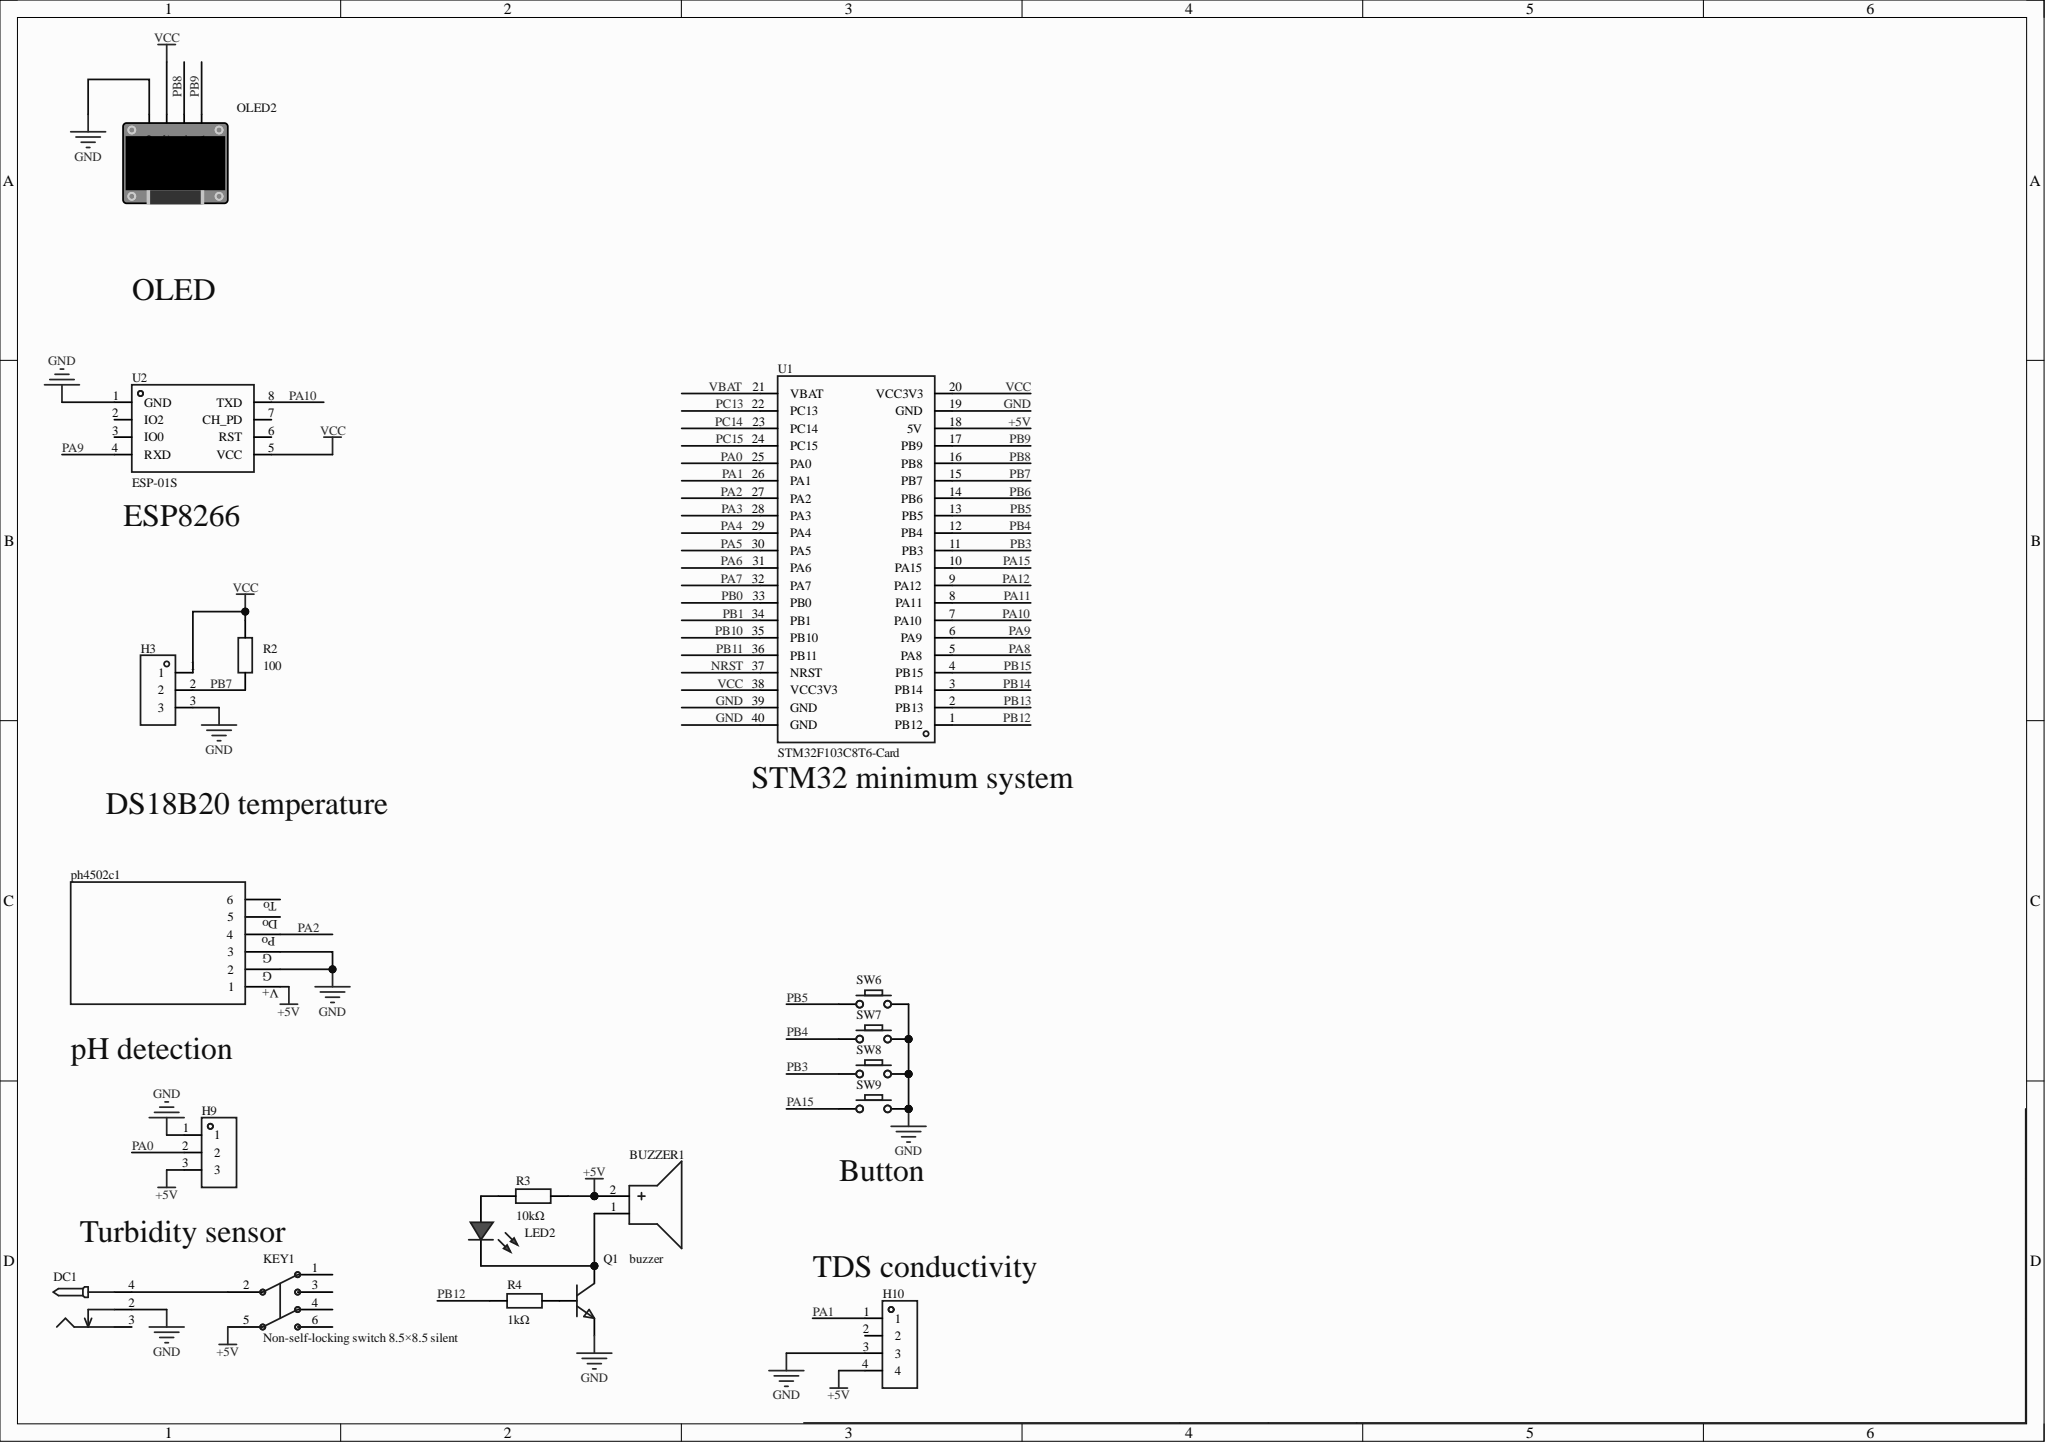Circuit board | Altium Designer | 19 parts | 20 nets
Bill of materials:
Comment,Description,Designator,Footprint,LibRef,Quantity
"buzzer","","BUZZER1","BUZ-TH_BD12.0-P6.00-D0.9-RD","buzzer","1"
"","","DC1","DC-2.0","DC-005_2.0","1"
"","","H3, H9","HDR-TH_3P-P2.54-V-F","HDR-F_2.54_1x3P","2"
"","","H10","HDR-TH_4P-P2.54-V-F","HDR-F_2.54_1x4P","1"
"Non-self-locking switch 8.5×8.5 silent","6脚，8.5×8.5","KEY1","SW-TH_6P-L8.5-W8.5-P2.54","无自锁开关 8.5×8.5 无声","1"
"","","LED2","LED_TH-3mm","LED_TH-R_3mm","1"
"","","OLED2","0.96OLED_4P","0.96OLED模块_4P","1"
"","","ph4502c1","PH4502C","PH4502C","1"
"","","Q1","S8050_TO_92","S8050_TO_NPN","1"
"100","","R2","Res_1/8W","Res_AXIAL-1/8W","1"
"10kΩ","","R3","Res_1/8W","Res_AXIAL-1/8W","1"
"1kΩ","","R4","Res_1/8W","Res_AXIAL-1/8W","1"
"","","SW6, SW7, SW8, SW9","Key_TH_3.5x6x4.3","Key_TH_3.5x6x4.3","4"
"STM32F103C8T6-Card","","U1","CONN-TH_L53.3-W22.9_STM32F103C8T6-CARD","STM32F103C8T6-Card","1"
"ESP-01S","","U2","WIFIM-TH_ESP-01S","ESP-01S_C111009","1"
Netlist (Protel format):
[
BUZZER1
BUZ-TH_BD12.0-P6.00-D0.9-RD
buzzer



]
[
DC1
DC-2.0




]
[
H3
HDR-TH_3P-P2.54-V-F




]
[
H9
HDR-TH_3P-P2.54-V-F




]
[
H10
HDR-TH_4P-P2.54-V-F




]
[
KEY1
SW-TH_6P-L8.5-W8.5-P2.54
Non-self-locking switch 8.5×8.5 silent



]
[
LED2
LED_TH-3mm




]
[
OLED2
0.96OLED_4P




]
[
ph4502c1
PH4502C




]
[
Q1
S8050_TO_92




]
[
R2
Res_1/8W
100



]
[
R3
Res_1/8W
10kΩ



]
[
R4
Res_1/8W
1kΩ



]
[
SW6
Key_TH_3.5x6x4.3




]
[
SW7
Key_TH_3.5x6x4.3




]
[
SW8
Key_TH_3.5x6x4.3




]
[
SW9
Key_TH_3.5x6x4.3




]
[
U1
CONN-TH_L53.3-W22.9_STM32F103C8T6-CARD
STM32F103C8T6-Card



]
[
U2
WIFIM-TH_ESP-01S
ESP-01S



]
(
VCC
H3-1
OLED2-2
R2-2
U1-20
U1-38
U2-5
)
(
PB12
R4-1
U1-1
)
(
PB9
OLED2-4
U1-17
)
(
PB8
OLED2-3
U1-16
)
(
PB7
H3-2
R2-1
U1-15
)
(
PB5
SW6-A
U1-13
)
(
PB4
SW7-A
U1-12
)
(
PB3
SW8-A
U1-11
)
(
PA15
SW9-A
U1-10
)
(
PA10
U1-7
U2-8
)
(
PA9
U1-6
U2-4
)
(
PA2
ph4502c1-4
U1-27
)
(
PA1
H10-1
U1-26
)
(
PA0
H9-2
U1-25
)
(
NetQ1_2
Q1-2
R4-2
)
(
NetLED2_1
LED2-1
R3-1
)
(
NetDC1_4
DC1-4
KEY1-2
)
(
NetBUZZER1_1
BUZZER1-1
LED2-2
Q1-3
)
(
GND
DC1-2
H3-3
H9-1
H10-3
OLED2-1
ph4502c1-2
ph4502c1-3
Q1-1
SW6-B
SW7-B
SW8-B
SW9-B
U1-19
U1-39
U1-40
U2-1
)
(
+5V
BUZZER1-2
H9-3
H10-4
KEY1-5
ph4502c1-1
R3-2
U1-18
)